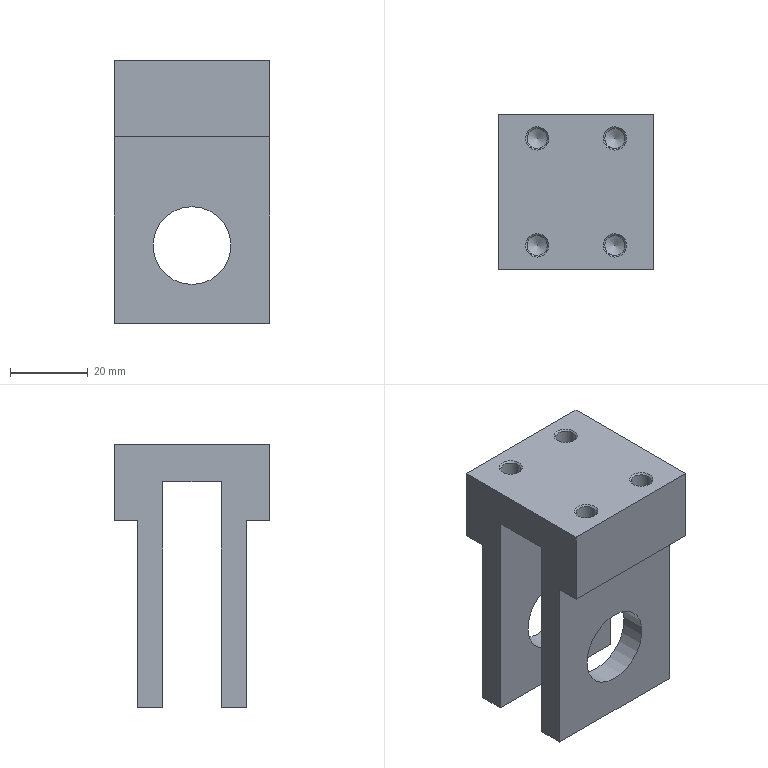Part | NX | features SIMPLE HOLE 5, DATUM_CSYS 4, SYMBOLIC_THREAD 4, SKETCH 3, EXTRUDE 2, HOLE PACKAGE 2 | 1 solid | 28 faces | box 40 x 40 x 67.571 mm | volume 44865 mm3 | plane 14 | cone 8 | cylinder 6 | commonest cylinder face diameters 5.2 x4 20 x2
STEP:
#1=CARTESIAN_POINT('',(-20.,-20.,4.571));
#2=VERTEX_POINT('',#1);
#3=CARTESIAN_POINT('',(-20.,-20.,-15.));
#4=VERTEX_POINT('',#3);
#5=CARTESIAN_POINT('',(-20.,-20.,0.));
#6=DIRECTION('',(0.,0.,-1.));
#7=VECTOR('',#6,1000.);
#8=LINE('',#5,#7);
#9=EDGE_CURVE('',#2,#4,#8,.T.);
#10=ORIENTED_EDGE('',*,*,#9,.T.);
#11=CARTESIAN_POINT('',(20.,-20.,-15.));
#12=VERTEX_POINT('',#11);
#13=CARTESIAN_POINT('',(20.,-20.,-15.));
#14=DIRECTION('',(-1.,0.,0.));
#15=VECTOR('',#14,1000.);
#16=LINE('',#13,#15);
#17=EDGE_CURVE('',#12,#4,#16,.T.);
#18=ORIENTED_EDGE('',*,*,#17,.F.);
#19=CARTESIAN_POINT('',(20.,-20.,4.571));
#20=VERTEX_POINT('',#19);
#21=CARTESIAN_POINT('',(20.,-20.,0.));
#22=DIRECTION('',(0.,0.,-1.));
#23=VECTOR('',#22,1000.);
#24=LINE('',#21,#23);
#25=EDGE_CURVE('',#20,#12,#24,.T.);
#26=ORIENTED_EDGE('',*,*,#25,.F.);
#27=CARTESIAN_POINT('',(-20.,-20.,4.571));
#28=DIRECTION('',(1.,0.,0.));
#29=VECTOR('',#28,1000.);
#30=LINE('',#27,#29);
#31=EDGE_CURVE('',#2,#20,#30,.T.);
#32=ORIENTED_EDGE('',*,*,#31,.F.);
#33=EDGE_LOOP('',(#10,#18,#26,#32));
#34=FACE_BOUND('',#33,.T.);
#35=CARTESIAN_POINT('',(20.,-20.,0.));
#36=DIRECTION('',(0.,1.,0.));
#37=DIRECTION('',(0.,0.,1.));
#38=AXIS2_PLACEMENT_3D('',#35,#36,#37);
#39=PLANE('',#38);
#40=ADVANCED_FACE('',(#34),#39,.F.);
#41=CARTESIAN_POINT('',(-20.,-14.,-15.));
#42=VERTEX_POINT('',#41);
#43=CARTESIAN_POINT('',(-20.,-20.,-15.));
#44=DIRECTION('',(0.,1.,0.));
#45=VECTOR('',#44,1000.);
#46=LINE('',#43,#45);
#47=EDGE_CURVE('',#4,#42,#46,.T.);
#48=ORIENTED_EDGE('',*,*,#47,.T.);
#49=CARTESIAN_POINT('',(20.,-14.,-15.));
#50=VERTEX_POINT('',#49);
#51=CARTESIAN_POINT('',(20.,-14.,-15.));
#52=DIRECTION('',(-1.,0.,0.));
#53=VECTOR('',#52,1000.);
#54=LINE('',#51,#53);
#55=EDGE_CURVE('',#50,#42,#54,.T.);
#56=ORIENTED_EDGE('',*,*,#55,.F.);
#57=CARTESIAN_POINT('',(20.,-20.,-15.));
#58=DIRECTION('',(0.,1.,0.));
#59=VECTOR('',#58,1000.);
#60=LINE('',#57,#59);
#61=EDGE_CURVE('',#12,#50,#60,.T.);
#62=ORIENTED_EDGE('',*,*,#61,.F.);
#63=ORIENTED_EDGE('',*,*,#17,.T.);
#64=EDGE_LOOP('',(#48,#56,#62,#63));
#65=FACE_BOUND('',#64,.T.);
#66=CARTESIAN_POINT('',(20.,-20.,-15.));
#67=DIRECTION('',(0.,0.,1.));
#68=DIRECTION('',(0.,-1.,0.));
#69=AXIS2_PLACEMENT_3D('',#66,#67,#68);
#70=PLANE('',#69);
#71=ADVANCED_FACE('',(#65),#70,.F.);
#72=CARTESIAN_POINT('',(0.,-14.,-33.));
#73=VERTEX_POINT('',#72);
#74=CARTESIAN_POINT('',(0.,-14.,-43.));
#75=DIRECTION('',(0.,1.,0.));
#76=DIRECTION('',(0.,0.,1.));
#77=AXIS2_PLACEMENT_3D('',#74,#75,#76);
#78=CIRCLE('',#77,10.);
#79=EDGE_CURVE('',#73,#73,#78,.T.);
#80=ORIENTED_EDGE('',*,*,#79,.T.);
#81=EDGE_LOOP('',(#80));
#82=FACE_BOUND('',#81,.T.);
#83=CARTESIAN_POINT('',(-20.,-14.,-63.));
#84=VERTEX_POINT('',#83);
#85=CARTESIAN_POINT('',(-20.,-14.,-15.));
#86=DIRECTION('',(0.,0.,-1.));
#87=VECTOR('',#86,1000.);
#88=LINE('',#85,#87);
#89=EDGE_CURVE('',#42,#84,#88,.T.);
#90=ORIENTED_EDGE('',*,*,#89,.T.);
#91=CARTESIAN_POINT('',(20.,-14.,-63.));
#92=VERTEX_POINT('',#91);
#93=CARTESIAN_POINT('',(20.,-14.,-63.));
#94=DIRECTION('',(-1.,0.,0.));
#95=VECTOR('',#94,1000.);
#96=LINE('',#93,#95);
#97=EDGE_CURVE('',#92,#84,#96,.T.);
#98=ORIENTED_EDGE('',*,*,#97,.F.);
#99=CARTESIAN_POINT('',(20.,-14.,-15.));
#100=DIRECTION('',(0.,0.,-1.));
#101=VECTOR('',#100,1000.);
#102=LINE('',#99,#101);
#103=EDGE_CURVE('',#50,#92,#102,.T.);
#104=ORIENTED_EDGE('',*,*,#103,.F.);
#105=ORIENTED_EDGE('',*,*,#55,.T.);
#106=EDGE_LOOP('',(#90,#98,#104,#105));
#107=FACE_BOUND('',#106,.T.);
#108=CARTESIAN_POINT('',(20.,-14.,-15.));
#109=DIRECTION('',(0.,1.,0.));
#110=DIRECTION('',(0.,0.,1.));
#111=AXIS2_PLACEMENT_3D('',#108,#109,#110);
#112=PLANE('',#111);
#113=ADVANCED_FACE('',(#82,#107),#112,.F.);
#114=CARTESIAN_POINT('',(-20.,-7.5,-63.));
#115=VERTEX_POINT('',#114);
#116=CARTESIAN_POINT('',(-20.,-14.,-63.));
#117=DIRECTION('',(0.,1.,0.));
#118=VECTOR('',#117,1000.);
#119=LINE('',#116,#118);
#120=EDGE_CURVE('',#84,#115,#119,.T.);
#121=ORIENTED_EDGE('',*,*,#120,.T.);
#122=CARTESIAN_POINT('',(20.,-7.5,-63.));
#123=VERTEX_POINT('',#122);
#124=CARTESIAN_POINT('',(20.,-7.5,-63.));
#125=DIRECTION('',(-1.,0.,0.));
#126=VECTOR('',#125,1000.);
#127=LINE('',#124,#126);
#128=EDGE_CURVE('',#123,#115,#127,.T.);
#129=ORIENTED_EDGE('',*,*,#128,.F.);
#130=CARTESIAN_POINT('',(20.,-14.,-63.));
#131=DIRECTION('',(0.,1.,0.));
#132=VECTOR('',#131,1000.);
#133=LINE('',#130,#132);
#134=EDGE_CURVE('',#92,#123,#133,.T.);
#135=ORIENTED_EDGE('',*,*,#134,.F.);
#136=ORIENTED_EDGE('',*,*,#97,.T.);
#137=EDGE_LOOP('',(#121,#129,#135,#136));
#138=FACE_BOUND('',#137,.T.);
#139=CARTESIAN_POINT('',(20.,-14.,-63.));
#140=DIRECTION('',(0.,0.,1.));
#141=DIRECTION('',(0.,-1.,0.));
#142=AXIS2_PLACEMENT_3D('',#139,#140,#141);
#143=PLANE('',#142);
#144=ADVANCED_FACE('',(#138),#143,.F.);
#145=CARTESIAN_POINT('',(0.,-7.5,-53.));
#146=VERTEX_POINT('',#145);
#147=CARTESIAN_POINT('',(0.,-7.5,-43.));
#148=DIRECTION('',(0.,-1.,0.));
#149=DIRECTION('',(0.,0.,-1.));
#150=AXIS2_PLACEMENT_3D('',#147,#148,#149);
#151=CIRCLE('',#150,10.);
#152=EDGE_CURVE('',#146,#146,#151,.T.);
#153=ORIENTED_EDGE('',*,*,#152,.T.);
#154=EDGE_LOOP('',(#153));
#155=FACE_BOUND('',#154,.T.);
#156=CARTESIAN_POINT('',(-20.,-7.5,-5.));
#157=VERTEX_POINT('',#156);
#158=CARTESIAN_POINT('',(-20.,-7.5,-63.));
#159=DIRECTION('',(0.,0.,1.));
#160=VECTOR('',#159,1000.);
#161=LINE('',#158,#160);
#162=EDGE_CURVE('',#115,#157,#161,.T.);
#163=ORIENTED_EDGE('',*,*,#162,.T.);
#164=CARTESIAN_POINT('',(20.,-7.5,-5.));
#165=VERTEX_POINT('',#164);
#166=CARTESIAN_POINT('',(20.,-7.5,-5.));
#167=DIRECTION('',(-1.,0.,0.));
#168=VECTOR('',#167,1000.);
#169=LINE('',#166,#168);
#170=EDGE_CURVE('',#165,#157,#169,.T.);
#171=ORIENTED_EDGE('',*,*,#170,.F.);
#172=CARTESIAN_POINT('',(20.,-7.5,-63.));
#173=DIRECTION('',(0.,0.,1.));
#174=VECTOR('',#173,1000.);
#175=LINE('',#172,#174);
#176=EDGE_CURVE('',#123,#165,#175,.T.);
#177=ORIENTED_EDGE('',*,*,#176,.F.);
#178=ORIENTED_EDGE('',*,*,#128,.T.);
#179=EDGE_LOOP('',(#163,#171,#177,#178));
#180=FACE_BOUND('',#179,.T.);
#181=CARTESIAN_POINT('',(20.,-7.5,-63.));
#182=DIRECTION('',(0.,-1.,0.));
#183=DIRECTION('',(0.,0.,-1.));
#184=AXIS2_PLACEMENT_3D('',#181,#182,#183);
#185=PLANE('',#184);
#186=ADVANCED_FACE('',(#155,#180),#185,.F.);
#187=CARTESIAN_POINT('',(-20.,7.5,-5.));
#188=VERTEX_POINT('',#187);
#189=CARTESIAN_POINT('',(-20.,-7.5,-5.));
#190=DIRECTION('',(0.,1.,0.));
#191=VECTOR('',#190,1000.);
#192=LINE('',#189,#191);
#193=EDGE_CURVE('',#157,#188,#192,.T.);
#194=ORIENTED_EDGE('',*,*,#193,.T.);
#195=CARTESIAN_POINT('',(20.,7.5,-5.));
#196=VERTEX_POINT('',#195);
#197=CARTESIAN_POINT('',(20.,7.5,-5.));
#198=DIRECTION('',(-1.,0.,0.));
#199=VECTOR('',#198,1000.);
#200=LINE('',#197,#199);
#201=EDGE_CURVE('',#196,#188,#200,.T.);
#202=ORIENTED_EDGE('',*,*,#201,.F.);
#203=CARTESIAN_POINT('',(20.,-7.5,-5.));
#204=DIRECTION('',(0.,1.,0.));
#205=VECTOR('',#204,1000.);
#206=LINE('',#203,#205);
#207=EDGE_CURVE('',#165,#196,#206,.T.);
#208=ORIENTED_EDGE('',*,*,#207,.F.);
#209=ORIENTED_EDGE('',*,*,#170,.T.);
#210=EDGE_LOOP('',(#194,#202,#208,#209));
#211=FACE_BOUND('',#210,.T.);
#212=CARTESIAN_POINT('',(20.,-7.5,-5.));
#213=DIRECTION('',(0.,0.,1.));
#214=DIRECTION('',(0.,-1.,0.));
#215=AXIS2_PLACEMENT_3D('',#212,#213,#214);
#216=PLANE('',#215);
#217=ADVANCED_FACE('',(#211),#216,.F.);
#218=CARTESIAN_POINT('',(0.,7.5,-33.));
#219=VERTEX_POINT('',#218);
#220=CARTESIAN_POINT('',(0.,7.5,-43.));
#221=DIRECTION('',(0.,1.,0.));
#222=DIRECTION('',(0.,0.,1.));
#223=AXIS2_PLACEMENT_3D('',#220,#221,#222);
#224=CIRCLE('',#223,10.);
#225=EDGE_CURVE('',#219,#219,#224,.T.);
#226=ORIENTED_EDGE('',*,*,#225,.T.);
#227=EDGE_LOOP('',(#226));
#228=FACE_BOUND('',#227,.T.);
#229=CARTESIAN_POINT('',(-20.,7.5,-63.));
#230=VERTEX_POINT('',#229);
#231=CARTESIAN_POINT('',(-20.,7.5,-5.));
#232=DIRECTION('',(0.,0.,-1.));
#233=VECTOR('',#232,1000.);
#234=LINE('',#231,#233);
#235=EDGE_CURVE('',#188,#230,#234,.T.);
#236=ORIENTED_EDGE('',*,*,#235,.T.);
#237=CARTESIAN_POINT('',(20.,7.5,-63.));
#238=VERTEX_POINT('',#237);
#239=CARTESIAN_POINT('',(20.,7.5,-63.));
#240=DIRECTION('',(-1.,0.,0.));
#241=VECTOR('',#240,1000.);
#242=LINE('',#239,#241);
#243=EDGE_CURVE('',#238,#230,#242,.T.);
#244=ORIENTED_EDGE('',*,*,#243,.F.);
#245=CARTESIAN_POINT('',(20.,7.5,-5.));
#246=DIRECTION('',(0.,0.,-1.));
#247=VECTOR('',#246,1000.);
#248=LINE('',#245,#247);
#249=EDGE_CURVE('',#196,#238,#248,.T.);
#250=ORIENTED_EDGE('',*,*,#249,.F.);
#251=ORIENTED_EDGE('',*,*,#201,.T.);
#252=EDGE_LOOP('',(#236,#244,#250,#251));
#253=FACE_BOUND('',#252,.T.);
#254=CARTESIAN_POINT('',(20.,7.5,-5.));
#255=DIRECTION('',(0.,1.,0.));
#256=DIRECTION('',(0.,0.,1.));
#257=AXIS2_PLACEMENT_3D('',#254,#255,#256);
#258=PLANE('',#257);
#259=ADVANCED_FACE('',(#228,#253),#258,.F.);
#260=CARTESIAN_POINT('',(-20.,14.,-63.));
#261=VERTEX_POINT('',#260);
#262=CARTESIAN_POINT('',(-20.,7.5,-63.));
#263=DIRECTION('',(0.,1.,0.));
#264=VECTOR('',#263,1000.);
#265=LINE('',#262,#264);
#266=EDGE_CURVE('',#230,#261,#265,.T.);
#267=ORIENTED_EDGE('',*,*,#266,.T.);
#268=CARTESIAN_POINT('',(20.,14.,-63.));
#269=VERTEX_POINT('',#268);
#270=CARTESIAN_POINT('',(20.,14.,-63.));
#271=DIRECTION('',(-1.,0.,0.));
#272=VECTOR('',#271,1000.);
#273=LINE('',#270,#272);
#274=EDGE_CURVE('',#269,#261,#273,.T.);
#275=ORIENTED_EDGE('',*,*,#274,.F.);
#276=CARTESIAN_POINT('',(20.,7.5,-63.));
#277=DIRECTION('',(0.,1.,0.));
#278=VECTOR('',#277,1000.);
#279=LINE('',#276,#278);
#280=EDGE_CURVE('',#238,#269,#279,.T.);
#281=ORIENTED_EDGE('',*,*,#280,.F.);
#282=ORIENTED_EDGE('',*,*,#243,.T.);
#283=EDGE_LOOP('',(#267,#275,#281,#282));
#284=FACE_BOUND('',#283,.T.);
#285=CARTESIAN_POINT('',(20.,7.5,-63.));
#286=DIRECTION('',(0.,0.,1.));
#287=DIRECTION('',(0.,-1.,0.));
#288=AXIS2_PLACEMENT_3D('',#285,#286,#287);
#289=PLANE('',#288);
#290=ADVANCED_FACE('',(#284),#289,.F.);
#291=CARTESIAN_POINT('',(0.,14.,-53.));
#292=VERTEX_POINT('',#291);
#293=CARTESIAN_POINT('',(0.,14.,-43.));
#294=DIRECTION('',(0.,-1.,0.));
#295=DIRECTION('',(0.,0.,-1.));
#296=AXIS2_PLACEMENT_3D('',#293,#294,#295);
#297=CIRCLE('',#296,10.);
#298=EDGE_CURVE('',#292,#292,#297,.T.);
#299=ORIENTED_EDGE('',*,*,#298,.T.);
#300=EDGE_LOOP('',(#299));
#301=FACE_BOUND('',#300,.T.);
#302=CARTESIAN_POINT('',(-20.,14.,-15.));
#303=VERTEX_POINT('',#302);
#304=CARTESIAN_POINT('',(-20.,14.,-63.));
#305=DIRECTION('',(0.,0.,1.));
#306=VECTOR('',#305,1000.);
#307=LINE('',#304,#306);
#308=EDGE_CURVE('',#261,#303,#307,.T.);
#309=ORIENTED_EDGE('',*,*,#308,.T.);
#310=CARTESIAN_POINT('',(20.,14.,-15.));
#311=VERTEX_POINT('',#310);
#312=CARTESIAN_POINT('',(20.,14.,-15.));
#313=DIRECTION('',(-1.,0.,0.));
#314=VECTOR('',#313,1000.);
#315=LINE('',#312,#314);
#316=EDGE_CURVE('',#311,#303,#315,.T.);
#317=ORIENTED_EDGE('',*,*,#316,.F.);
#318=CARTESIAN_POINT('',(20.,14.,-63.));
#319=DIRECTION('',(0.,0.,1.));
#320=VECTOR('',#319,1000.);
#321=LINE('',#318,#320);
#322=EDGE_CURVE('',#269,#311,#321,.T.);
#323=ORIENTED_EDGE('',*,*,#322,.F.);
#324=ORIENTED_EDGE('',*,*,#274,.T.);
#325=EDGE_LOOP('',(#309,#317,#323,#324));
#326=FACE_BOUND('',#325,.T.);
#327=CARTESIAN_POINT('',(20.,14.,-63.));
#328=DIRECTION('',(0.,-1.,0.));
#329=DIRECTION('',(0.,0.,-1.));
#330=AXIS2_PLACEMENT_3D('',#327,#328,#329);
#331=PLANE('',#330);
#332=ADVANCED_FACE('',(#301,#326),#331,.F.);
#333=CARTESIAN_POINT('',(-20.,20.,-15.));
#334=VERTEX_POINT('',#333);
#335=CARTESIAN_POINT('',(-20.,14.,-15.));
#336=DIRECTION('',(0.,1.,0.));
#337=VECTOR('',#336,1000.);
#338=LINE('',#335,#337);
#339=EDGE_CURVE('',#303,#334,#338,.T.);
#340=ORIENTED_EDGE('',*,*,#339,.T.);
#341=CARTESIAN_POINT('',(20.,20.,-15.));
#342=VERTEX_POINT('',#341);
#343=CARTESIAN_POINT('',(20.,20.,-15.));
#344=DIRECTION('',(-1.,0.,0.));
#345=VECTOR('',#344,1000.);
#346=LINE('',#343,#345);
#347=EDGE_CURVE('',#342,#334,#346,.T.);
#348=ORIENTED_EDGE('',*,*,#347,.F.);
#349=CARTESIAN_POINT('',(20.,14.,-15.));
#350=DIRECTION('',(0.,1.,0.));
#351=VECTOR('',#350,1000.);
#352=LINE('',#349,#351);
#353=EDGE_CURVE('',#311,#342,#352,.T.);
#354=ORIENTED_EDGE('',*,*,#353,.F.);
#355=ORIENTED_EDGE('',*,*,#316,.T.);
#356=EDGE_LOOP('',(#340,#348,#354,#355));
#357=FACE_BOUND('',#356,.T.);
#358=CARTESIAN_POINT('',(20.,14.,-15.));
#359=DIRECTION('',(0.,0.,1.));
#360=DIRECTION('',(0.,-1.,0.));
#361=AXIS2_PLACEMENT_3D('',#358,#359,#360);
#362=PLANE('',#361);
#363=ADVANCED_FACE('',(#357),#362,.F.);
#364=CARTESIAN_POINT('',(-20.,20.,4.571));
#365=VERTEX_POINT('',#364);
#366=CARTESIAN_POINT('',(-20.,20.,-15.));
#367=DIRECTION('',(0.,0.,1.));
#368=VECTOR('',#367,1000.);
#369=LINE('',#366,#368);
#370=EDGE_CURVE('',#334,#365,#369,.T.);
#371=ORIENTED_EDGE('',*,*,#370,.T.);
#372=CARTESIAN_POINT('',(20.,20.,4.571));
#373=VERTEX_POINT('',#372);
#374=CARTESIAN_POINT('',(20.,20.,4.571));
#375=DIRECTION('',(-1.,0.,0.));
#376=VECTOR('',#375,1000.);
#377=LINE('',#374,#376);
#378=EDGE_CURVE('',#373,#365,#377,.T.);
#379=ORIENTED_EDGE('',*,*,#378,.F.);
#380=CARTESIAN_POINT('',(20.,20.,-15.));
#381=DIRECTION('',(0.,0.,1.));
#382=VECTOR('',#381,1000.);
#383=LINE('',#380,#382);
#384=EDGE_CURVE('',#342,#373,#383,.T.);
#385=ORIENTED_EDGE('',*,*,#384,.F.);
#386=ORIENTED_EDGE('',*,*,#347,.T.);
#387=EDGE_LOOP('',(#371,#379,#385,#386));
#388=FACE_BOUND('',#387,.T.);
#389=CARTESIAN_POINT('',(20.,20.,-15.));
#390=DIRECTION('',(0.,-1.,0.));
#391=DIRECTION('',(0.,0.,-1.));
#392=AXIS2_PLACEMENT_3D('',#389,#390,#391);
#393=PLANE('',#392);
#394=ADVANCED_FACE('',(#388),#393,.F.);
#395=ORIENTED_EDGE('',*,*,#25,.T.);
#396=ORIENTED_EDGE('',*,*,#61,.T.);
#397=ORIENTED_EDGE('',*,*,#103,.T.);
#398=ORIENTED_EDGE('',*,*,#134,.T.);
#399=ORIENTED_EDGE('',*,*,#176,.T.);
#400=ORIENTED_EDGE('',*,*,#207,.T.);
#401=ORIENTED_EDGE('',*,*,#249,.T.);
#402=ORIENTED_EDGE('',*,*,#280,.T.);
#403=ORIENTED_EDGE('',*,*,#322,.T.);
#404=ORIENTED_EDGE('',*,*,#353,.T.);
#405=ORIENTED_EDGE('',*,*,#384,.T.);
#406=CARTESIAN_POINT('',(20.,-20.,4.571));
#407=DIRECTION('',(0.,1.,0.));
#408=VECTOR('',#407,1000.);
#409=LINE('',#406,#408);
#410=EDGE_CURVE('',#20,#373,#409,.T.);
#411=ORIENTED_EDGE('',*,*,#410,.F.);
#412=EDGE_LOOP('',(#395,#396,#397,#398,#399,#400,#401,#402,#403,#404,#405,#411));
#413=FACE_BOUND('',#412,.T.);
#414=CARTESIAN_POINT('',(20.,0.,0.));
#415=DIRECTION('',(1.,0.,0.));
#416=DIRECTION('',(0.,0.,-1.));
#417=AXIS2_PLACEMENT_3D('',#414,#415,#416);
#418=PLANE('',#417);
#419=ADVANCED_FACE('',(#413),#418,.T.);
#420=ORIENTED_EDGE('',*,*,#9,.F.);
#421=CARTESIAN_POINT('',(-20.,20.,4.571));
#422=DIRECTION('',(0.,-1.,0.));
#423=VECTOR('',#422,1000.);
#424=LINE('',#421,#423);
#425=EDGE_CURVE('',#365,#2,#424,.T.);
#426=ORIENTED_EDGE('',*,*,#425,.F.);
#427=ORIENTED_EDGE('',*,*,#370,.F.);
#428=ORIENTED_EDGE('',*,*,#339,.F.);
#429=ORIENTED_EDGE('',*,*,#308,.F.);
#430=ORIENTED_EDGE('',*,*,#266,.F.);
#431=ORIENTED_EDGE('',*,*,#235,.F.);
#432=ORIENTED_EDGE('',*,*,#193,.F.);
#433=ORIENTED_EDGE('',*,*,#162,.F.);
#434=ORIENTED_EDGE('',*,*,#120,.F.);
#435=ORIENTED_EDGE('',*,*,#89,.F.);
#436=ORIENTED_EDGE('',*,*,#47,.F.);
#437=EDGE_LOOP('',(#420,#426,#427,#428,#429,#430,#431,#432,#433,#434,#435,#436));
#438=FACE_BOUND('',#437,.T.);
#439=CARTESIAN_POINT('',(-20.,0.,0.));
#440=DIRECTION('',(1.,0.,0.));
#441=DIRECTION('',(0.,0.,-1.));
#442=AXIS2_PLACEMENT_3D('',#439,#440,#441);
#443=PLANE('',#442);
#444=ADVANCED_FACE('',(#438),#443,.F.);
#445=ORIENTED_EDGE('',*,*,#298,.F.);
#446=EDGE_LOOP('',(#445));
#447=FACE_BOUND('',#446,.T.);
#448=ORIENTED_EDGE('',*,*,#225,.F.);
#449=EDGE_LOOP('',(#448));
#450=FACE_BOUND('',#449,.T.);
#451=CARTESIAN_POINT('',(0.,-14.,-43.));
#452=DIRECTION('',(0.,1.,0.));
#453=DIRECTION('',(0.,0.,1.));
#454=AXIS2_PLACEMENT_3D('',#451,#452,#453);
#455=CYLINDRICAL_SURFACE('',#454,10.);
#456=ADVANCED_FACE('',(#447,#450),#455,.F.);
#457=ORIENTED_EDGE('',*,*,#79,.F.);
#458=EDGE_LOOP('',(#457));
#459=FACE_BOUND('',#458,.T.);
#460=ORIENTED_EDGE('',*,*,#152,.F.);
#461=EDGE_LOOP('',(#460));
#462=FACE_BOUND('',#461,.T.);
#463=CARTESIAN_POINT('',(0.,-14.,-43.));
#464=DIRECTION('',(0.,1.,0.));
#465=DIRECTION('',(0.,0.,1.));
#466=AXIS2_PLACEMENT_3D('',#463,#464,#465);
#467=CYLINDRICAL_SURFACE('',#466,10.);
#468=ADVANCED_FACE('',(#459,#462),#467,.F.);
#469=CARTESIAN_POINT('',(10.,10.75,4.571));
#470=VERTEX_POINT('',#469);
#471=CARTESIAN_POINT('',(10.,13.75,4.571));
#472=DIRECTION('',(0.,0.,1.));
#473=DIRECTION('',(0.,-1.,0.));
#474=AXIS2_PLACEMENT_3D('',#471,#472,#473);
#475=CIRCLE('',#474,3.);
#476=EDGE_CURVE('',#470,#470,#475,.F.);
#477=ORIENTED_EDGE('',*,*,#476,.T.);
#478=EDGE_LOOP('',(#477));
#479=FACE_BOUND('',#478,.T.);
#480=CARTESIAN_POINT('',(10.,-16.75,4.571));
#481=VERTEX_POINT('',#480);
#482=CARTESIAN_POINT('',(10.,-13.75,4.571));
#483=DIRECTION('',(0.,0.,1.));
#484=DIRECTION('',(0.,-1.,0.));
#485=AXIS2_PLACEMENT_3D('',#482,#483,#484);
#486=CIRCLE('',#485,3.);
#487=EDGE_CURVE('',#481,#481,#486,.F.);
#488=ORIENTED_EDGE('',*,*,#487,.T.);
#489=EDGE_LOOP('',(#488));
#490=FACE_BOUND('',#489,.T.);
#491=CARTESIAN_POINT('',(-10.,10.75,4.571));
#492=VERTEX_POINT('',#491);
#493=CARTESIAN_POINT('',(-10.,13.75,4.571));
#494=DIRECTION('',(0.,0.,1.));
#495=DIRECTION('',(0.,-1.,0.));
#496=AXIS2_PLACEMENT_3D('',#493,#494,#495);
#497=CIRCLE('',#496,3.);
#498=EDGE_CURVE('',#492,#492,#497,.F.);
#499=ORIENTED_EDGE('',*,*,#498,.T.);
#500=EDGE_LOOP('',(#499));
#501=FACE_BOUND('',#500,.T.);
#502=CARTESIAN_POINT('',(-10.,-16.75,4.571));
#503=VERTEX_POINT('',#502);
#504=CARTESIAN_POINT('',(-10.,-13.75,4.571));
#505=DIRECTION('',(0.,0.,1.));
#506=DIRECTION('',(0.,-1.,0.));
#507=AXIS2_PLACEMENT_3D('',#504,#505,#506);
#508=CIRCLE('',#507,3.);
#509=EDGE_CURVE('',#503,#503,#508,.F.);
#510=ORIENTED_EDGE('',*,*,#509,.T.);
#511=EDGE_LOOP('',(#510));
#512=FACE_BOUND('',#511,.T.);
#513=ORIENTED_EDGE('',*,*,#425,.T.);
#514=ORIENTED_EDGE('',*,*,#31,.T.);
#515=ORIENTED_EDGE('',*,*,#410,.T.);
#516=ORIENTED_EDGE('',*,*,#378,.T.);
#517=EDGE_LOOP('',(#513,#514,#515,#516));
#518=FACE_BOUND('',#517,.T.);
#519=CARTESIAN_POINT('',(0.,0.,4.571));
#520=DIRECTION('',(0.,0.,1.));
#521=DIRECTION('',(0.,-1.,0.));
#522=AXIS2_PLACEMENT_3D('',#519,#520,#521);
#523=PLANE('',#522);
#524=ADVANCED_FACE('',(#479,#490,#501,#512,#518),#523,.T.);
#525=CARTESIAN_POINT('',(-10.,-11.15,-10.429));
#526=VERTEX_POINT('',#525);
#527=CARTESIAN_POINT('',(-10.,-13.75,-10.429));
#528=DIRECTION('',(0.,0.,-1.));
#529=DIRECTION('',(0.,1.,0.));
#530=AXIS2_PLACEMENT_3D('',#527,#528,#529);
#531=CIRCLE('',#530,2.6);
#532=EDGE_CURVE('',#526,#526,#531,.F.);
#533=ORIENTED_EDGE('',*,*,#532,.T.);
#534=EDGE_LOOP('',(#533));
#535=FACE_BOUND('',#534,.T.);
#536=CARTESIAN_POINT('',(-10.,-13.75,-11.991));
#537=VERTEX_POINT('',#536);
#538=VERTEX_LOOP('',#537);
#539=FACE_BOUND('',#538,.T.);
#540=CARTESIAN_POINT('',(-10.,-13.75,-10.429));
#541=DIRECTION('',(0.,0.,1.));
#542=DIRECTION('',(0.,-1.,0.));
#543=AXIS2_PLACEMENT_3D('',#540,#541,#542);
#544=CONICAL_SURFACE('',#543,2.6,1.03);
#545=ADVANCED_FACE('',(#535,#539),#544,.F.);
#546=CARTESIAN_POINT('',(-7.4,-13.75,4.171));
#547=VERTEX_POINT('',#546);
#548=CARTESIAN_POINT('',(-10.,-13.75,4.171));
#549=DIRECTION('',(0.,0.,1.));
#550=DIRECTION('',(1.,0.,0.));
#551=AXIS2_PLACEMENT_3D('',#548,#549,#550);
#552=CIRCLE('',#551,2.6);
#553=EDGE_CURVE('',#547,#547,#552,.T.);
#554=ORIENTED_EDGE('',*,*,#553,.T.);
#555=EDGE_LOOP('',(#554));
#556=FACE_BOUND('',#555,.T.);
#557=ORIENTED_EDGE('',*,*,#532,.F.);
#558=EDGE_LOOP('',(#557));
#559=FACE_BOUND('',#558,.T.);
#560=CARTESIAN_POINT('',(-10.,-13.75,4.571));
#561=DIRECTION('',(0.,0.,-1.));
#562=DIRECTION('',(0.,1.,0.));
#563=AXIS2_PLACEMENT_3D('',#560,#561,#562);
#564=CYLINDRICAL_SURFACE('',#563,2.6);
#565=ADVANCED_FACE('',(#556,#559),#564,.F.);
#566=ORIENTED_EDGE('',*,*,#553,.F.);
#567=EDGE_LOOP('',(#566));
#568=FACE_BOUND('',#567,.T.);
#569=ORIENTED_EDGE('',*,*,#509,.F.);
#570=EDGE_LOOP('',(#569));
#571=FACE_BOUND('',#570,.T.);
#572=CARTESIAN_POINT('',(-10.,-13.75,4.571));
#573=DIRECTION('',(0.,0.,1.));
#574=DIRECTION('',(1.,0.,0.));
#575=AXIS2_PLACEMENT_3D('',#572,#573,#574);
#576=CONICAL_SURFACE('',#575,3.,0.7854);
#577=ADVANCED_FACE('',(#568,#571),#576,.F.);
#578=CARTESIAN_POINT('',(-10.,16.35,-10.429));
#579=VERTEX_POINT('',#578);
#580=CARTESIAN_POINT('',(-10.,13.75,-10.429));
#581=DIRECTION('',(0.,0.,-1.));
#582=DIRECTION('',(0.,1.,0.));
#583=AXIS2_PLACEMENT_3D('',#580,#581,#582);
#584=CIRCLE('',#583,2.6);
#585=EDGE_CURVE('',#579,#579,#584,.F.);
#586=ORIENTED_EDGE('',*,*,#585,.T.);
#587=EDGE_LOOP('',(#586));
#588=FACE_BOUND('',#587,.T.);
#589=CARTESIAN_POINT('',(-10.,13.75,-11.991));
#590=VERTEX_POINT('',#589);
#591=VERTEX_LOOP('',#590);
#592=FACE_BOUND('',#591,.T.);
#593=CARTESIAN_POINT('',(-10.,13.75,-10.429));
#594=DIRECTION('',(0.,0.,1.));
#595=DIRECTION('',(0.,-1.,0.));
#596=AXIS2_PLACEMENT_3D('',#593,#594,#595);
#597=CONICAL_SURFACE('',#596,2.6,1.03);
#598=ADVANCED_FACE('',(#588,#592),#597,.F.);
#599=CARTESIAN_POINT('',(-7.4,13.75,4.171));
#600=VERTEX_POINT('',#599);
#601=CARTESIAN_POINT('',(-10.,13.75,4.171));
#602=DIRECTION('',(0.,0.,1.));
#603=DIRECTION('',(1.,0.,0.));
#604=AXIS2_PLACEMENT_3D('',#601,#602,#603);
#605=CIRCLE('',#604,2.6);
#606=EDGE_CURVE('',#600,#600,#605,.T.);
#607=ORIENTED_EDGE('',*,*,#606,.T.);
#608=EDGE_LOOP('',(#607));
#609=FACE_BOUND('',#608,.T.);
#610=ORIENTED_EDGE('',*,*,#585,.F.);
#611=EDGE_LOOP('',(#610));
#612=FACE_BOUND('',#611,.T.);
#613=CARTESIAN_POINT('',(-10.,13.75,4.571));
#614=DIRECTION('',(0.,0.,-1.));
#615=DIRECTION('',(0.,1.,0.));
#616=AXIS2_PLACEMENT_3D('',#613,#614,#615);
#617=CYLINDRICAL_SURFACE('',#616,2.6);
#618=ADVANCED_FACE('',(#609,#612),#617,.F.);
#619=ORIENTED_EDGE('',*,*,#606,.F.);
#620=EDGE_LOOP('',(#619));
#621=FACE_BOUND('',#620,.T.);
#622=ORIENTED_EDGE('',*,*,#498,.F.);
#623=EDGE_LOOP('',(#622));
#624=FACE_BOUND('',#623,.T.);
#625=CARTESIAN_POINT('',(-10.,13.75,4.571));
#626=DIRECTION('',(0.,0.,1.));
#627=DIRECTION('',(1.,0.,0.));
#628=AXIS2_PLACEMENT_3D('',#625,#626,#627);
#629=CONICAL_SURFACE('',#628,3.,0.7854);
#630=ADVANCED_FACE('',(#621,#624),#629,.F.);
#631=CARTESIAN_POINT('',(10.,-11.15,-10.429));
#632=VERTEX_POINT('',#631);
#633=CARTESIAN_POINT('',(10.,-13.75,-10.429));
#634=DIRECTION('',(0.,0.,-1.));
#635=DIRECTION('',(0.,1.,0.));
#636=AXIS2_PLACEMENT_3D('',#633,#634,#635);
#637=CIRCLE('',#636,2.6);
#638=EDGE_CURVE('',#632,#632,#637,.F.);
#639=ORIENTED_EDGE('',*,*,#638,.T.);
#640=EDGE_LOOP('',(#639));
#641=FACE_BOUND('',#640,.T.);
#642=CARTESIAN_POINT('',(10.,-13.75,-11.991));
#643=VERTEX_POINT('',#642);
#644=VERTEX_LOOP('',#643);
#645=FACE_BOUND('',#644,.T.);
#646=CARTESIAN_POINT('',(10.,-13.75,-10.429));
#647=DIRECTION('',(0.,0.,1.));
#648=DIRECTION('',(0.,-1.,0.));
#649=AXIS2_PLACEMENT_3D('',#646,#647,#648);
#650=CONICAL_SURFACE('',#649,2.6,1.03);
#651=ADVANCED_FACE('',(#641,#645),#650,.F.);
#652=CARTESIAN_POINT('',(12.6,-13.75,4.171));
#653=VERTEX_POINT('',#652);
#654=CARTESIAN_POINT('',(10.,-13.75,4.171));
#655=DIRECTION('',(0.,0.,1.));
#656=DIRECTION('',(1.,0.,0.));
#657=AXIS2_PLACEMENT_3D('',#654,#655,#656);
#658=CIRCLE('',#657,2.6);
#659=EDGE_CURVE('',#653,#653,#658,.T.);
#660=ORIENTED_EDGE('',*,*,#659,.T.);
#661=EDGE_LOOP('',(#660));
#662=FACE_BOUND('',#661,.T.);
#663=ORIENTED_EDGE('',*,*,#638,.F.);
#664=EDGE_LOOP('',(#663));
#665=FACE_BOUND('',#664,.T.);
#666=CARTESIAN_POINT('',(10.,-13.75,4.571));
#667=DIRECTION('',(0.,0.,-1.));
#668=DIRECTION('',(0.,1.,0.));
#669=AXIS2_PLACEMENT_3D('',#666,#667,#668);
#670=CYLINDRICAL_SURFACE('',#669,2.6);
#671=ADVANCED_FACE('',(#662,#665),#670,.F.);
#672=ORIENTED_EDGE('',*,*,#659,.F.);
#673=EDGE_LOOP('',(#672));
#674=FACE_BOUND('',#673,.T.);
#675=ORIENTED_EDGE('',*,*,#487,.F.);
#676=EDGE_LOOP('',(#675));
#677=FACE_BOUND('',#676,.T.);
#678=CARTESIAN_POINT('',(10.,-13.75,4.571));
#679=DIRECTION('',(0.,0.,1.));
#680=DIRECTION('',(1.,0.,0.));
#681=AXIS2_PLACEMENT_3D('',#678,#679,#680);
#682=CONICAL_SURFACE('',#681,3.,0.7854);
#683=ADVANCED_FACE('',(#674,#677),#682,.F.);
#684=CARTESIAN_POINT('',(10.,16.35,-10.429));
#685=VERTEX_POINT('',#684);
#686=CARTESIAN_POINT('',(10.,13.75,-10.429));
#687=DIRECTION('',(0.,0.,-1.));
#688=DIRECTION('',(0.,1.,0.));
#689=AXIS2_PLACEMENT_3D('',#686,#687,#688);
#690=CIRCLE('',#689,2.6);
#691=EDGE_CURVE('',#685,#685,#690,.F.);
#692=ORIENTED_EDGE('',*,*,#691,.T.);
#693=EDGE_LOOP('',(#692));
#694=FACE_BOUND('',#693,.T.);
#695=CARTESIAN_POINT('',(10.,13.75,-11.991));
#696=VERTEX_POINT('',#695);
#697=VERTEX_LOOP('',#696);
#698=FACE_BOUND('',#697,.T.);
#699=CARTESIAN_POINT('',(10.,13.75,-10.429));
#700=DIRECTION('',(0.,0.,1.));
#701=DIRECTION('',(0.,-1.,0.));
#702=AXIS2_PLACEMENT_3D('',#699,#700,#701);
#703=CONICAL_SURFACE('',#702,2.6,1.03);
#704=ADVANCED_FACE('',(#694,#698),#703,.F.);
#705=CARTESIAN_POINT('',(12.6,13.75,4.171));
#706=VERTEX_POINT('',#705);
#707=CARTESIAN_POINT('',(10.,13.75,4.171));
#708=DIRECTION('',(0.,0.,1.));
#709=DIRECTION('',(1.,0.,0.));
#710=AXIS2_PLACEMENT_3D('',#707,#708,#709);
#711=CIRCLE('',#710,2.6);
#712=EDGE_CURVE('',#706,#706,#711,.T.);
#713=ORIENTED_EDGE('',*,*,#712,.T.);
#714=EDGE_LOOP('',(#713));
#715=FACE_BOUND('',#714,.T.);
#716=ORIENTED_EDGE('',*,*,#691,.F.);
#717=EDGE_LOOP('',(#716));
#718=FACE_BOUND('',#717,.T.);
#719=CARTESIAN_POINT('',(10.,13.75,4.571));
#720=DIRECTION('',(0.,0.,-1.));
#721=DIRECTION('',(0.,1.,0.));
#722=AXIS2_PLACEMENT_3D('',#719,#720,#721);
#723=CYLINDRICAL_SURFACE('',#722,2.6);
#724=ADVANCED_FACE('',(#715,#718),#723,.F.);
#725=ORIENTED_EDGE('',*,*,#712,.F.);
#726=EDGE_LOOP('',(#725));
#727=FACE_BOUND('',#726,.T.);
#728=ORIENTED_EDGE('',*,*,#476,.F.);
#729=EDGE_LOOP('',(#728));
#730=FACE_BOUND('',#729,.T.);
#731=CARTESIAN_POINT('',(10.,13.75,4.571));
#732=DIRECTION('',(0.,0.,1.));
#733=DIRECTION('',(1.,0.,0.));
#734=AXIS2_PLACEMENT_3D('',#731,#732,#733);
#735=CONICAL_SURFACE('',#734,3.,0.7854);
#736=ADVANCED_FACE('',(#727,#730),#735,.F.);
#737=CLOSED_SHELL('',(#40,#71,#113,#144,#186,#217,#259,#290,#332,#363,#394,#419,#444,#456,#468,#524,#545,#565,#577,#598,#618,#630,#651,#671,#683,#704,#724,#736));
#738=MANIFOLD_SOLID_BREP('',#737);
#739=(LENGTH_UNIT()NAMED_UNIT(*)SI_UNIT(.MILLI.,.METRE.));
#740=UNCERTAINTY_MEASURE_WITH_UNIT(LENGTH_MEASURE(0.00001),#739,'','');
#741=(NAMED_UNIT(*)PLANE_ANGLE_UNIT()SI_UNIT($,.RADIAN.));
#742=(NAMED_UNIT(*)SI_UNIT($,.STERADIAN.)SOLID_ANGLE_UNIT());
#743=(GEOMETRIC_REPRESENTATION_CONTEXT(3)GLOBAL_UNCERTAINTY_ASSIGNED_CONTEXT((#740))GLOBAL_UNIT_ASSIGNED_CONTEXT((#739,#741,#742))REPRESENTATION_CONTEXT('',''));
#744=ADVANCED_BREP_SHAPE_REPRESENTATION('',(#738),#743);